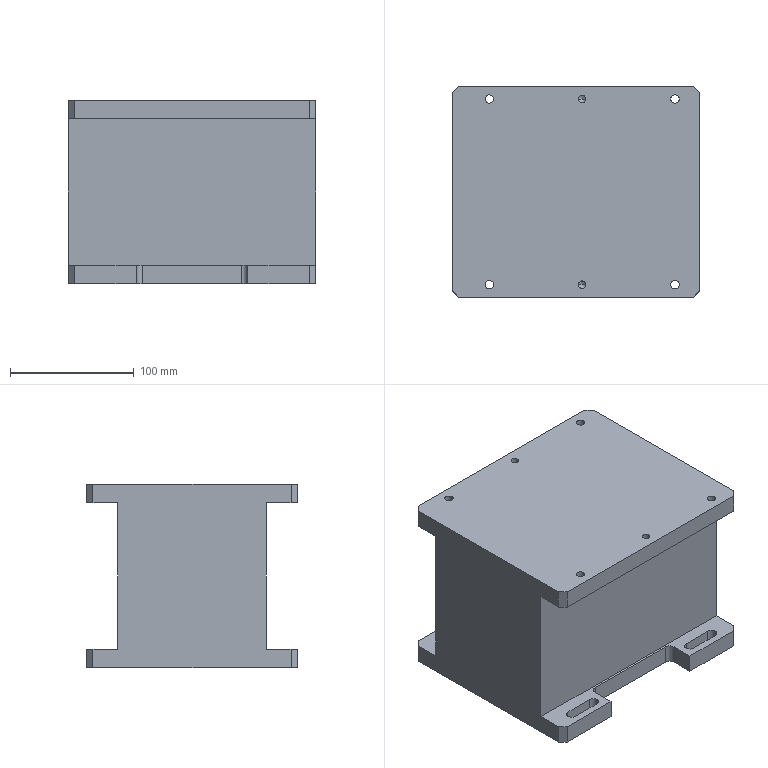Part | STEP file | 11-FG-SB00111 | 1 solid | 64 faces | box 200 x 170 x 148.5 mm | volume 3812542 mm3 | plane 34 | cylinder 26 | cone 4 | commonest cylinder face diameters 8.5 x12 6.8 x8 6 x4 10 x2